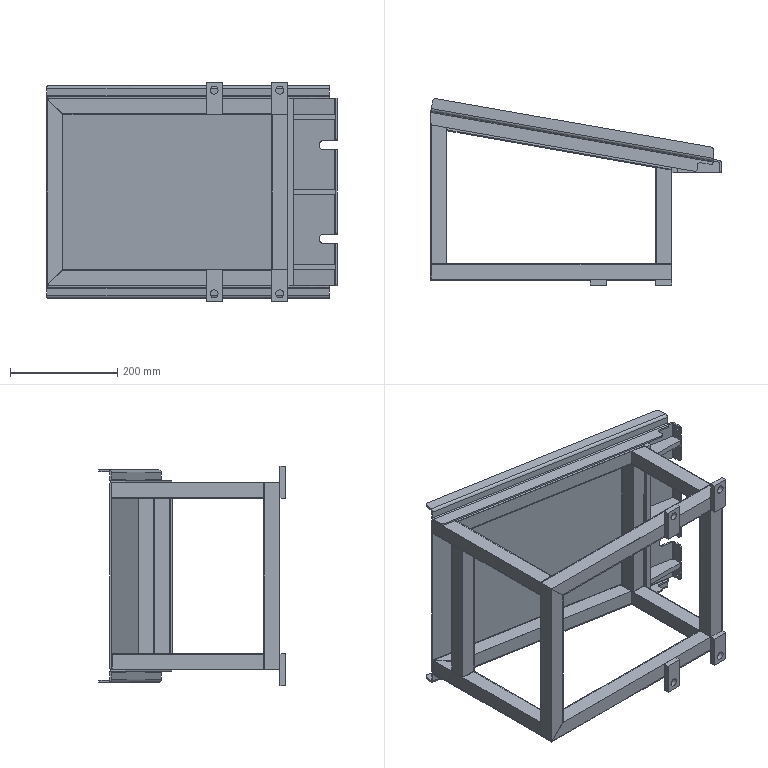Part | NX | features guide rail pipe_Default_As Machined_ 24 | 23 solids | 255 faces | box 542.513 x 348.38 x 410 mm | volume 1580217 mm3 | plane 213 | cylinder 42 | commonest cylinder face diameters 10 x27 4 x7 15 x4 6.5 x2 18 x2